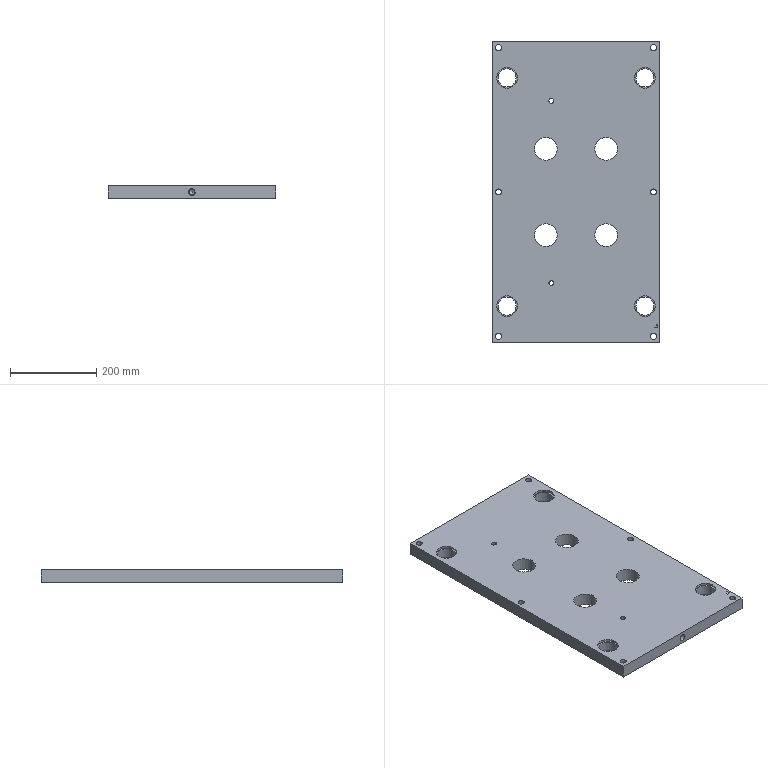Part | NX | features 模具.stp<1>[10] 2 | 1 solid | 69 faces | box 390 x 700 x 30 mm | volume 7689695 mm3 | cylinder 34 | plane 33 | cone 2 | commonest cylinder face diameters 14 x6 20 x6 42 x4 48 x4 53 x4 11 x2